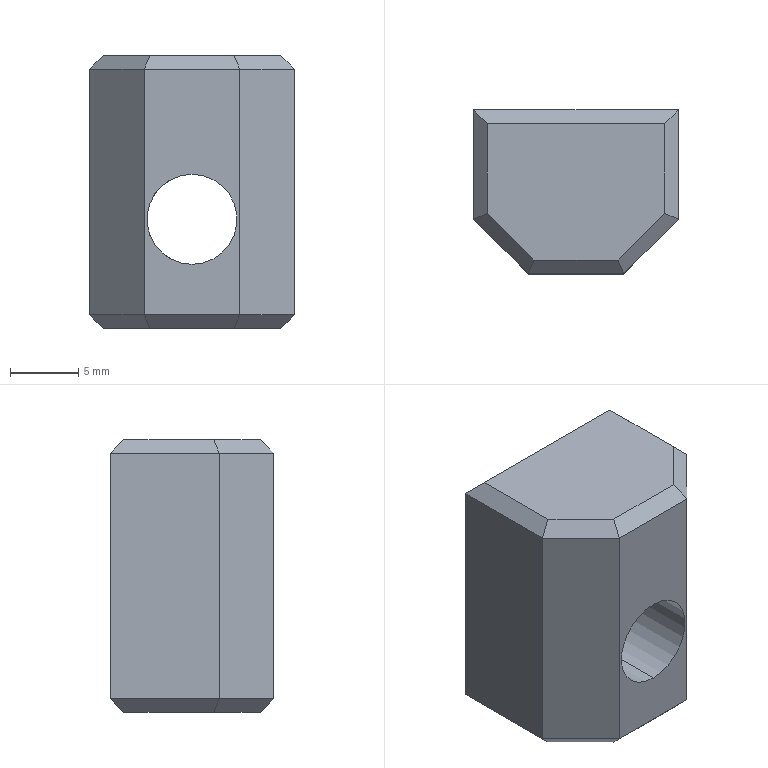Part | Creo | 1 solid | 25 faces | box 15 x 12 x 20 mm | volume 2397 mm3 | plane 21 | cylinder 4 | commonest cylinder face diameters 6.6 x2 11 x2
STEP:
#1=CARTESIAN_POINT('',(0.,0.,0.));
#2=DIRECTION('',(0.,0.,1.));
#3=DIRECTION('',(1.,0.,0.));
#4=AXIS2_PLACEMENT_3D('',#1,#2,#3);
#5=CARTESIAN_POINT('',(-37.05,242.414,-34.767));
#6=VERTEX_POINT('',#5);
#7=CARTESIAN_POINT('',(-40.464,239.,-34.767));
#8=VERTEX_POINT('',#7);
#9=CARTESIAN_POINT('',(-37.05,242.414,-34.767));
#10=DIRECTION('',(-0.7071,-0.7071,0.));
#11=VECTOR('',#10,4.828);
#12=LINE('',#9,#11);
#13=EDGE_CURVE('',#6,#8,#12,.T.);
#14=ORIENTED_EDGE('',*,*,#13,.F.);
#15=CARTESIAN_POINT('',(-37.05,249.,-34.767));
#16=VERTEX_POINT('',#15);
#17=CARTESIAN_POINT('',(-37.05,242.414,-34.767));
#18=DIRECTION('',(0.,1.,0.));
#19=VECTOR('',#18,6.586);
#20=LINE('',#17,#19);
#21=EDGE_CURVE('',#6,#16,#20,.T.);
#22=ORIENTED_EDGE('',*,*,#21,.T.);
#23=CARTESIAN_POINT('',(-50.05,249.,-34.767));
#24=VERTEX_POINT('',#23);
#25=CARTESIAN_POINT('',(-37.05,249.,-34.767));
#26=DIRECTION('',(-1.,0.,0.));
#27=VECTOR('',#26,13.);
#28=LINE('',#25,#27);
#29=EDGE_CURVE('',#16,#24,#28,.T.);
#30=ORIENTED_EDGE('',*,*,#29,.T.);
#31=CARTESIAN_POINT('',(-50.05,242.414,-34.767));
#32=VERTEX_POINT('',#31);
#33=CARTESIAN_POINT('',(-50.05,249.,-34.767));
#34=DIRECTION('',(0.,-1.,0.));
#35=VECTOR('',#34,6.586);
#36=LINE('',#33,#35);
#37=EDGE_CURVE('',#24,#32,#36,.T.);
#38=ORIENTED_EDGE('',*,*,#37,.T.);
#39=CARTESIAN_POINT('',(-46.636,239.,-34.767));
#40=VERTEX_POINT('',#39);
#41=CARTESIAN_POINT('',(-46.636,239.,-34.767));
#42=DIRECTION('',(-0.7071,0.7071,0.));
#43=VECTOR('',#42,4.828);
#44=LINE('',#41,#43);
#45=EDGE_CURVE('',#40,#32,#44,.T.);
#46=ORIENTED_EDGE('',*,*,#45,.F.);
#47=CARTESIAN_POINT('',(-46.636,239.,-34.767));
#48=DIRECTION('',(1.,0.,0.));
#49=VECTOR('',#48,6.172);
#50=LINE('',#47,#49);
#51=EDGE_CURVE('',#40,#8,#50,.T.);
#52=ORIENTED_EDGE('',*,*,#51,.T.);
#53=EDGE_LOOP('',(#14,#22,#30,#38,#46,#52));
#54=FACE_OUTER_BOUND('',#53,.F.);
#55=CARTESIAN_POINT('',(-36.05,250.,-34.767));
#56=DIRECTION('',(0.,0.,-1.));
#57=DIRECTION('',(0.,1.,0.));
#58=AXIS2_PLACEMENT_3D('',#55,#56,#57);
#59=PLANE('',#58);
#60=ADVANCED_FACE('',(#54),#59,.T.);
#61=CARTESIAN_POINT('',(-40.05,238.,-33.767));
#62=VERTEX_POINT('',#61);
#63=CARTESIAN_POINT('',(-40.464,239.,-34.767));
#64=DIRECTION('',(0.2811,-0.6786,0.6786));
#65=VECTOR('',#64,1.474);
#66=LINE('',#63,#65);
#67=EDGE_CURVE('',#8,#62,#66,.T.);
#68=ORIENTED_EDGE('',*,*,#67,.T.);
#69=CARTESIAN_POINT('',(-36.05,242.,-33.767));
#70=VERTEX_POINT('',#69);
#71=CARTESIAN_POINT('',(-36.05,242.,-33.767));
#72=DIRECTION('',(-0.7071,-0.7071,0.));
#73=VECTOR('',#72,5.657);
#74=LINE('',#71,#73);
#75=EDGE_CURVE('',#70,#62,#74,.T.);
#76=ORIENTED_EDGE('',*,*,#75,.F.);
#77=CARTESIAN_POINT('',(-36.05,242.,-33.767));
#78=DIRECTION('',(-0.6786,0.2811,-0.6786));
#79=VECTOR('',#78,1.474);
#80=LINE('',#77,#79);
#81=EDGE_CURVE('',#70,#6,#80,.T.);
#82=ORIENTED_EDGE('',*,*,#81,.T.);
#83=ORIENTED_EDGE('',*,*,#13,.T.);
#84=EDGE_LOOP('',(#68,#76,#82,#83));
#85=FACE_OUTER_BOUND('',#84,.F.);
#86=CARTESIAN_POINT('',(-40.05,238.,-33.767));
#87=DIRECTION('',(0.5,-0.5,-0.7071));
#88=DIRECTION('',(-0.7071,-0.7071,0.));
#89=AXIS2_PLACEMENT_3D('',#86,#87,#88);
#90=PLANE('',#89);
#91=ADVANCED_FACE('',(#85),#90,.T.);
#92=CARTESIAN_POINT('',(-47.05,238.,-33.767));
#93=VERTEX_POINT('',#92);
#94=CARTESIAN_POINT('',(-46.636,239.,-34.767));
#95=DIRECTION('',(-0.2811,-0.6786,0.6786));
#96=VECTOR('',#95,1.474);
#97=LINE('',#94,#96);
#98=EDGE_CURVE('',#40,#93,#97,.T.);
#99=ORIENTED_EDGE('',*,*,#98,.T.);
#100=CARTESIAN_POINT('',(-40.05,238.,-33.767));
#101=DIRECTION('',(-1.,0.,0.));
#102=VECTOR('',#101,7.);
#103=LINE('',#100,#102);
#104=EDGE_CURVE('',#62,#93,#103,.T.);
#105=ORIENTED_EDGE('',*,*,#104,.F.);
#106=ORIENTED_EDGE('',*,*,#67,.F.);
#107=ORIENTED_EDGE('',*,*,#51,.F.);
#108=EDGE_LOOP('',(#99,#105,#106,#107));
#109=FACE_OUTER_BOUND('',#108,.F.);
#110=CARTESIAN_POINT('',(-36.05,239.,-34.767));
#111=DIRECTION('',(0.,0.7071,0.7071));
#112=DIRECTION('',(-1.,0.,0.));
#113=AXIS2_PLACEMENT_3D('',#110,#111,#112);
#114=PLANE('',#113);
#115=ADVANCED_FACE('',(#109),#114,.F.);
#116=CARTESIAN_POINT('',(-51.05,242.,-33.767));
#117=VERTEX_POINT('',#116);
#118=CARTESIAN_POINT('',(-50.05,242.414,-34.767));
#119=DIRECTION('',(-0.6786,-0.2811,0.6786));
#120=VECTOR('',#119,1.474);
#121=LINE('',#118,#120);
#122=EDGE_CURVE('',#32,#117,#121,.T.);
#123=ORIENTED_EDGE('',*,*,#122,.T.);
#124=CARTESIAN_POINT('',(-47.05,238.,-33.767));
#125=DIRECTION('',(-0.7071,0.7071,0.));
#126=VECTOR('',#125,5.657);
#127=LINE('',#124,#126);
#128=EDGE_CURVE('',#93,#117,#127,.T.);
#129=ORIENTED_EDGE('',*,*,#128,.F.);
#130=ORIENTED_EDGE('',*,*,#98,.F.);
#131=ORIENTED_EDGE('',*,*,#45,.T.);
#132=EDGE_LOOP('',(#123,#129,#130,#131));
#133=FACE_OUTER_BOUND('',#132,.F.);
#134=CARTESIAN_POINT('',(-47.05,238.,-33.767));
#135=DIRECTION('',(-0.5,-0.5,-0.7071));
#136=DIRECTION('',(-0.7071,0.7071,0.));
#137=AXIS2_PLACEMENT_3D('',#134,#135,#136);
#138=PLANE('',#137);
#139=ADVANCED_FACE('',(#133),#138,.T.);
#140=CARTESIAN_POINT('',(-51.05,250.,-33.767));
#141=VERTEX_POINT('',#140);
#142=CARTESIAN_POINT('',(-51.05,250.,-33.767));
#143=DIRECTION('',(0.5774,-0.5774,-0.5774));
#144=VECTOR('',#143,1.732);
#145=LINE('',#142,#144);
#146=EDGE_CURVE('',#141,#24,#145,.T.);
#147=ORIENTED_EDGE('',*,*,#146,.F.);
#148=CARTESIAN_POINT('',(-51.05,242.,-33.767));
#149=DIRECTION('',(0.,1.,0.));
#150=VECTOR('',#149,8.);
#151=LINE('',#148,#150);
#152=EDGE_CURVE('',#117,#141,#151,.T.);
#153=ORIENTED_EDGE('',*,*,#152,.F.);
#154=ORIENTED_EDGE('',*,*,#122,.F.);
#155=ORIENTED_EDGE('',*,*,#37,.F.);
#156=EDGE_LOOP('',(#147,#153,#154,#155));
#157=FACE_OUTER_BOUND('',#156,.F.);
#158=CARTESIAN_POINT('',(-51.05,250.,-33.767));
#159=DIRECTION('',(0.7071,0.,0.7071));
#160=DIRECTION('',(0.,-1.,0.));
#161=AXIS2_PLACEMENT_3D('',#158,#159,#160);
#162=PLANE('',#161);
#163=ADVANCED_FACE('',(#157),#162,.F.);
#164=ORIENTED_EDGE('',*,*,#146,.T.);
#165=ORIENTED_EDGE('',*,*,#29,.F.);
#166=CARTESIAN_POINT('',(-36.05,250.,-33.767));
#167=VERTEX_POINT('',#166);
#168=CARTESIAN_POINT('',(-36.05,250.,-33.767));
#169=DIRECTION('',(-0.5774,-0.5774,-0.5774));
#170=VECTOR('',#169,1.732);
#171=LINE('',#168,#170);
#172=EDGE_CURVE('',#167,#16,#171,.T.);
#173=ORIENTED_EDGE('',*,*,#172,.F.);
#174=CARTESIAN_POINT('',(-51.05,250.,-33.767));
#175=DIRECTION('',(1.,0.,0.));
#176=VECTOR('',#175,15.);
#177=LINE('',#174,#176);
#178=EDGE_CURVE('',#141,#167,#177,.T.);
#179=ORIENTED_EDGE('',*,*,#178,.F.);
#180=EDGE_LOOP('',(#164,#165,#173,#179));
#181=FACE_OUTER_BOUND('',#180,.F.);
#182=CARTESIAN_POINT('',(50.05,250.,-33.767));
#183=DIRECTION('',(0.,0.7071,-0.7071));
#184=DIRECTION('',(1.,0.,0.));
#185=AXIS2_PLACEMENT_3D('',#182,#183,#184);
#186=PLANE('',#185);
#187=ADVANCED_FACE('',(#181),#186,.T.);
#188=ORIENTED_EDGE('',*,*,#172,.T.);
#189=ORIENTED_EDGE('',*,*,#21,.F.);
#190=ORIENTED_EDGE('',*,*,#81,.F.);
#191=CARTESIAN_POINT('',(-36.05,250.,-33.767));
#192=DIRECTION('',(0.,-1.,0.));
#193=VECTOR('',#192,8.);
#194=LINE('',#191,#193);
#195=EDGE_CURVE('',#167,#70,#194,.T.);
#196=ORIENTED_EDGE('',*,*,#195,.F.);
#197=EDGE_LOOP('',(#188,#189,#190,#196));
#198=FACE_OUTER_BOUND('',#197,.F.);
#199=CARTESIAN_POINT('',(-37.05,250.,-34.767));
#200=DIRECTION('',(-0.7071,0.,0.7071));
#201=DIRECTION('',(0.,-1.,0.));
#202=AXIS2_PLACEMENT_3D('',#199,#200,#201);
#203=PLANE('',#202);
#204=ADVANCED_FACE('',(#198),#203,.F.);
#205=CARTESIAN_POINT('',(-36.05,242.,-15.767));
#206=VERTEX_POINT('',#205);
#207=CARTESIAN_POINT('',(-36.05,242.,-15.767));
#208=DIRECTION('',(0.,0.,-1.));
#209=VECTOR('',#208,18.);
#210=LINE('',#207,#209);
#211=EDGE_CURVE('',#206,#70,#210,.T.);
#212=ORIENTED_EDGE('',*,*,#211,.F.);
#213=CARTESIAN_POINT('',(-36.05,250.,-15.767));
#214=VERTEX_POINT('',#213);
#215=CARTESIAN_POINT('',(-36.05,242.,-15.767));
#216=DIRECTION('',(0.,1.,0.));
#217=VECTOR('',#216,8.);
#218=LINE('',#215,#217);
#219=EDGE_CURVE('',#206,#214,#218,.T.);
#220=ORIENTED_EDGE('',*,*,#219,.T.);
#221=CARTESIAN_POINT('',(-36.05,250.,-33.767));
#222=DIRECTION('',(0.,0.,1.));
#223=VECTOR('',#222,18.);
#224=LINE('',#221,#223);
#225=EDGE_CURVE('',#167,#214,#224,.T.);
#226=ORIENTED_EDGE('',*,*,#225,.F.);
#227=ORIENTED_EDGE('',*,*,#195,.T.);
#228=EDGE_LOOP('',(#212,#220,#226,#227));
#229=FACE_OUTER_BOUND('',#228,.F.);
#230=CARTESIAN_POINT('',(-36.05,250.,-14.767));
#231=DIRECTION('',(1.,0.,0.));
#232=DIRECTION('',(0.,0.,-1.));
#233=AXIS2_PLACEMENT_3D('',#230,#231,#232);
#234=PLANE('',#233);
#235=ADVANCED_FACE('',(#229),#234,.T.);
#236=ORIENTED_EDGE('',*,*,#211,.T.);
#237=ORIENTED_EDGE('',*,*,#75,.T.);
#238=CARTESIAN_POINT('',(-40.05,238.,-15.767));
#239=VERTEX_POINT('',#238);
#240=CARTESIAN_POINT('',(-40.05,238.,-33.767));
#241=DIRECTION('',(0.,0.,1.));
#242=VECTOR('',#241,18.);
#243=LINE('',#240,#242);
#244=EDGE_CURVE('',#62,#239,#243,.T.);
#245=ORIENTED_EDGE('',*,*,#244,.T.);
#246=CARTESIAN_POINT('',(-40.05,238.,-15.767));
#247=DIRECTION('',(0.7071,0.7071,0.));
#248=VECTOR('',#247,5.657);
#249=LINE('',#246,#248);
#250=EDGE_CURVE('',#239,#206,#249,.T.);
#251=ORIENTED_EDGE('',*,*,#250,.T.);
#252=EDGE_LOOP('',(#236,#237,#245,#251));
#253=FACE_OUTER_BOUND('',#252,.F.);
#254=CARTESIAN_POINT('',(-40.05,238.,8.06));
#255=DIRECTION('',(-0.7071,0.7071,0.));
#256=DIRECTION('',(0.,0.,-1.));
#257=AXIS2_PLACEMENT_3D('',#254,#255,#256);
#258=PLANE('',#257);
#259=ADVANCED_FACE('',(#253),#258,.F.);
#260=ORIENTED_EDGE('',*,*,#244,.F.);
#261=ORIENTED_EDGE('',*,*,#104,.T.);
#262=CARTESIAN_POINT('',(-47.05,238.,-15.767));
#263=VERTEX_POINT('',#262);
#264=CARTESIAN_POINT('',(-47.05,238.,-15.767));
#265=DIRECTION('',(0.,0.,-1.));
#266=VECTOR('',#265,18.);
#267=LINE('',#264,#266);
#268=EDGE_CURVE('',#263,#93,#267,.T.);
#269=ORIENTED_EDGE('',*,*,#268,.F.);
#270=CARTESIAN_POINT('',(-47.05,238.,-15.767));
#271=DIRECTION('',(1.,0.,0.));
#272=VECTOR('',#271,7.);
#273=LINE('',#270,#272);
#274=EDGE_CURVE('',#263,#239,#273,.T.);
#275=ORIENTED_EDGE('',*,*,#274,.T.);
#276=EDGE_LOOP('',(#260,#261,#269,#275));
#277=FACE_OUTER_BOUND('',#276,.F.);
#278=CARTESIAN_POINT('',(-43.55,238.,-30.067));
#279=VERTEX_POINT('',#278);
#280=CARTESIAN_POINT('',(-43.55,238.,-23.467));
#281=VERTEX_POINT('',#280);
#282=CARTESIAN_POINT('',(-43.55,238.,-26.767));
#283=DIRECTION('',(0.,1.,0.));
#284=DIRECTION('',(0.,0.,-1.));
#285=AXIS2_PLACEMENT_3D('',#282,#283,#284);
#286=CIRCLE('',#285,3.3);
#287=EDGE_CURVE('',#279,#281,#286,.T.);
#288=ORIENTED_EDGE('',*,*,#287,.F.);
#289=CARTESIAN_POINT('',(-43.55,238.,-26.767));
#290=DIRECTION('',(0.,1.,0.));
#291=DIRECTION('',(0.,0.,1.));
#292=AXIS2_PLACEMENT_3D('',#289,#290,#291);
#293=CIRCLE('',#292,3.3);
#294=EDGE_CURVE('',#281,#279,#293,.T.);
#295=ORIENTED_EDGE('',*,*,#294,.F.);
#296=EDGE_LOOP('',(#288,#295));
#297=FACE_BOUND('',#296,.F.);
#298=CARTESIAN_POINT('',(50.05,238.,8.06));
#299=DIRECTION('',(0.,-1.,0.));
#300=DIRECTION('',(0.,0.,-1.));
#301=AXIS2_PLACEMENT_3D('',#298,#299,#300);
#302=PLANE('',#301);
#303=ADVANCED_FACE('',(#277,#297),#302,.T.);
#304=CARTESIAN_POINT('',(-43.55,243.,-23.467));
#305=VERTEX_POINT('',#304);
#306=CARTESIAN_POINT('',(-46.85,243.,-26.767));
#307=VERTEX_POINT('',#306);
#308=CARTESIAN_POINT('',(-43.55,243.,-26.767));
#309=DIRECTION('',(0.,-1.,0.));
#310=DIRECTION('',(0.,0.,1.));
#311=AXIS2_PLACEMENT_3D('',#308,#309,#310);
#312=CIRCLE('',#311,3.3);
#313=EDGE_CURVE('',#305,#307,#312,.T.);
#314=ORIENTED_EDGE('',*,*,#313,.T.);
#315=CARTESIAN_POINT('',(-43.55,243.,-30.067));
#316=VERTEX_POINT('',#315);
#317=CARTESIAN_POINT('',(-43.55,243.,-26.767));
#318=DIRECTION('',(0.,-1.,0.));
#319=DIRECTION('',(-1.,0.,0.));
#320=AXIS2_PLACEMENT_3D('',#317,#318,#319);
#321=CIRCLE('',#320,3.3);
#322=EDGE_CURVE('',#307,#316,#321,.T.);
#323=ORIENTED_EDGE('',*,*,#322,.T.);
#324=CARTESIAN_POINT('',(-43.55,243.,-30.067));
#325=DIRECTION('',(0.,-1.,0.));
#326=VECTOR('',#325,5.);
#327=LINE('',#324,#326);
#328=EDGE_CURVE('',#316,#279,#327,.T.);
#329=ORIENTED_EDGE('',*,*,#328,.T.);
#330=ORIENTED_EDGE('',*,*,#287,.T.);
#331=CARTESIAN_POINT('',(-43.55,243.,-23.467));
#332=DIRECTION('',(0.,-1.,0.));
#333=VECTOR('',#332,5.);
#334=LINE('',#331,#333);
#335=EDGE_CURVE('',#305,#281,#334,.T.);
#336=ORIENTED_EDGE('',*,*,#335,.F.);
#337=EDGE_LOOP('',(#314,#323,#329,#330,#336));
#338=FACE_OUTER_BOUND('',#337,.F.);
#339=CARTESIAN_POINT('',(-43.55,50.,-26.767));
#340=DIRECTION('',(0.,-1.,0.));
#341=DIRECTION('',(0.,0.,-1.));
#342=AXIS2_PLACEMENT_3D('',#339,#340,#341);
#343=CYLINDRICAL_SURFACE('',#342,3.3);
#344=ADVANCED_FACE('',(#338),#343,.F.);
#345=CARTESIAN_POINT('',(-49.05,243.,-26.767));
#346=VERTEX_POINT('',#345);
#347=CARTESIAN_POINT('',(-43.55,243.,-21.267));
#348=VERTEX_POINT('',#347);
#349=CARTESIAN_POINT('',(-43.55,243.,-26.767));
#350=DIRECTION('',(0.,1.,0.));
#351=DIRECTION('',(-1.,0.,0.));
#352=AXIS2_PLACEMENT_3D('',#349,#350,#351);
#353=CIRCLE('',#352,5.5);
#354=EDGE_CURVE('',#346,#348,#353,.T.);
#355=ORIENTED_EDGE('',*,*,#354,.F.);
#356=CARTESIAN_POINT('',(-43.55,243.,-32.267));
#357=VERTEX_POINT('',#356);
#358=CARTESIAN_POINT('',(-43.55,243.,-26.767));
#359=DIRECTION('',(0.,1.,0.));
#360=DIRECTION('',(0.,0.,-1.));
#361=AXIS2_PLACEMENT_3D('',#358,#359,#360);
#362=CIRCLE('',#361,5.5);
#363=EDGE_CURVE('',#357,#346,#362,.T.);
#364=ORIENTED_EDGE('',*,*,#363,.F.);
#365=CARTESIAN_POINT('',(-38.05,243.,-26.767));
#366=VERTEX_POINT('',#365);
#367=CARTESIAN_POINT('',(-43.55,243.,-26.767));
#368=DIRECTION('',(0.,1.,0.));
#369=DIRECTION('',(1.,0.,0.));
#370=AXIS2_PLACEMENT_3D('',#367,#368,#369);
#371=CIRCLE('',#370,5.5);
#372=EDGE_CURVE('',#366,#357,#371,.T.);
#373=ORIENTED_EDGE('',*,*,#372,.F.);
#374=CARTESIAN_POINT('',(-43.55,243.,-26.767));
#375=DIRECTION('',(0.,1.,0.));
#376=DIRECTION('',(0.,0.,1.));
#377=AXIS2_PLACEMENT_3D('',#374,#375,#376);
#378=CIRCLE('',#377,5.5);
#379=EDGE_CURVE('',#348,#366,#378,.T.);
#380=ORIENTED_EDGE('',*,*,#379,.F.);
#381=EDGE_LOOP('',(#355,#364,#373,#380));
#382=FACE_OUTER_BOUND('',#381,.F.);
#383=ORIENTED_EDGE('',*,*,#322,.F.);
#384=ORIENTED_EDGE('',*,*,#313,.F.);
#385=CARTESIAN_POINT('',(-43.55,243.,-26.767));
#386=DIRECTION('',(0.,-1.,0.));
#387=DIRECTION('',(0.,0.,-1.));
#388=AXIS2_PLACEMENT_3D('',#385,#386,#387);
#389=CIRCLE('',#388,3.3);
#390=EDGE_CURVE('',#316,#305,#389,.T.);
#391=ORIENTED_EDGE('',*,*,#390,.F.);
#392=EDGE_LOOP('',(#383,#384,#391));
#393=FACE_BOUND('',#392,.F.);
#394=CARTESIAN_POINT('',(-43.55,243.,-21.267));
#395=DIRECTION('',(0.,-1.,0.));
#396=DIRECTION('',(1.,0.,0.));
#397=AXIS2_PLACEMENT_3D('',#394,#395,#396);
#398=PLANE('',#397);
#399=ADVANCED_FACE('',(#382,#393),#398,.F.);
#400=ORIENTED_EDGE('',*,*,#390,.T.);
#401=ORIENTED_EDGE('',*,*,#335,.T.);
#402=ORIENTED_EDGE('',*,*,#294,.T.);
#403=ORIENTED_EDGE('',*,*,#328,.F.);
#404=EDGE_LOOP('',(#400,#401,#402,#403));
#405=FACE_OUTER_BOUND('',#404,.F.);
#406=CARTESIAN_POINT('',(-43.55,50.,-26.767));
#407=DIRECTION('',(0.,-1.,0.));
#408=DIRECTION('',(0.,0.,-1.));
#409=AXIS2_PLACEMENT_3D('',#406,#407,#408);
#410=CYLINDRICAL_SURFACE('',#409,3.3);
#411=ADVANCED_FACE('',(#405),#410,.F.);
#412=CARTESIAN_POINT('',(-43.55,250.,-21.267));
#413=VERTEX_POINT('',#412);
#414=CARTESIAN_POINT('',(-43.55,250.,-32.267));
#415=VERTEX_POINT('',#414);
#416=CARTESIAN_POINT('',(-43.55,250.,-26.767));
#417=DIRECTION('',(0.,-1.,0.));
#418=DIRECTION('',(0.,0.,1.));
#419=AXIS2_PLACEMENT_3D('',#416,#417,#418);
#420=CIRCLE('',#419,5.5);
#421=EDGE_CURVE('',#413,#415,#420,.T.);
#422=ORIENTED_EDGE('',*,*,#421,.T.);
#423=CARTESIAN_POINT('',(-43.55,250.,-32.267));
#424=DIRECTION('',(0.,-1.,0.));
#425=VECTOR('',#424,7.);
#426=LINE('',#423,#425);
#427=EDGE_CURVE('',#415,#357,#426,.T.);
#428=ORIENTED_EDGE('',*,*,#427,.T.);
#429=ORIENTED_EDGE('',*,*,#363,.T.);
#430=ORIENTED_EDGE('',*,*,#354,.T.);
#431=CARTESIAN_POINT('',(-43.55,250.,-21.267));
#432=DIRECTION('',(0.,-1.,0.));
#433=VECTOR('',#432,7.);
#434=LINE('',#431,#433);
#435=EDGE_CURVE('',#413,#348,#434,.T.);
#436=ORIENTED_EDGE('',*,*,#435,.F.);
#437=EDGE_LOOP('',(#422,#428,#429,#430,#436));
#438=FACE_OUTER_BOUND('',#437,.F.);
#439=CARTESIAN_POINT('',(-43.55,250.,-26.767));
#440=DIRECTION('',(0.,-1.,0.));
#441=DIRECTION('',(0.,0.,-1.));
#442=AXIS2_PLACEMENT_3D('',#439,#440,#441);
#443=CYLINDRICAL_SURFACE('',#442,5.5);
#444=ADVANCED_FACE('',(#438),#443,.F.);
#445=CARTESIAN_POINT('',(-51.05,250.,-15.767));
#446=VERTEX_POINT('',#445);
#447=CARTESIAN_POINT('',(-51.05,250.,-15.767));
#448=DIRECTION('',(0.,0.,-1.));
#449=VECTOR('',#448,18.);
#450=LINE('',#447,#449);
#451=EDGE_CURVE('',#446,#141,#450,.T.);
#452=ORIENTED_EDGE('',*,*,#451,.T.);
#453=ORIENTED_EDGE('',*,*,#178,.T.);
#454=ORIENTED_EDGE('',*,*,#225,.T.);
#455=CARTESIAN_POINT('',(-36.05,250.,-15.767));
#456=DIRECTION('',(-1.,0.,0.));
#457=VECTOR('',#456,15.);
#458=LINE('',#455,#457);
#459=EDGE_CURVE('',#214,#446,#458,.T.);
#460=ORIENTED_EDGE('',*,*,#459,.T.);
#461=EDGE_LOOP('',(#452,#453,#454,#460));
#462=FACE_OUTER_BOUND('',#461,.F.);
#463=CARTESIAN_POINT('',(-43.55,250.,-26.767));
#464=DIRECTION('',(0.,-1.,0.));
#465=DIRECTION('',(0.,0.,-1.));
#466=AXIS2_PLACEMENT_3D('',#463,#464,#465);
#467=CIRCLE('',#466,5.5);
#468=EDGE_CURVE('',#415,#413,#467,.T.);
#469=ORIENTED_EDGE('',*,*,#468,.F.);
#470=ORIENTED_EDGE('',*,*,#421,.F.);
#471=EDGE_LOOP('',(#469,#470));
#472=FACE_BOUND('',#471,.F.);
#473=CARTESIAN_POINT('',(50.05,250.,8.06));
#474=DIRECTION('',(0.,-1.,0.));
#475=DIRECTION('',(0.,0.,-1.));
#476=AXIS2_PLACEMENT_3D('',#473,#474,#475);
#477=PLANE('',#476);
#478=ADVANCED_FACE('',(#462,#472),#477,.F.);
#479=ORIENTED_EDGE('',*,*,#468,.T.);
#480=ORIENTED_EDGE('',*,*,#435,.T.);
#481=ORIENTED_EDGE('',*,*,#379,.T.);
#482=ORIENTED_EDGE('',*,*,#372,.T.);
#483=ORIENTED_EDGE('',*,*,#427,.F.);
#484=EDGE_LOOP('',(#479,#480,#481,#482,#483));
#485=FACE_OUTER_BOUND('',#484,.F.);
#486=CARTESIAN_POINT('',(-43.55,250.,-26.767));
#487=DIRECTION('',(0.,-1.,0.));
#488=DIRECTION('',(0.,0.,-1.));
#489=AXIS2_PLACEMENT_3D('',#486,#487,#488);
#490=CYLINDRICAL_SURFACE('',#489,5.5);
#491=ADVANCED_FACE('',(#485),#490,.F.);
#492=ORIENTED_EDGE('',*,*,#451,.F.);
#493=CARTESIAN_POINT('',(-51.05,242.,-15.767));
#494=VERTEX_POINT('',#493);
#495=CARTESIAN_POINT('',(-51.05,250.,-15.767));
#496=DIRECTION('',(0.,-1.,0.));
#497=VECTOR('',#496,8.);
#498=LINE('',#495,#497);
#499=EDGE_CURVE('',#446,#494,#498,.T.);
#500=ORIENTED_EDGE('',*,*,#499,.T.);
#501=CARTESIAN_POINT('',(-51.05,242.,-33.767));
#502=DIRECTION('',(0.,0.,1.));
#503=VECTOR('',#502,18.);
#504=LINE('',#501,#503);
#505=EDGE_CURVE('',#117,#494,#504,.T.);
#506=ORIENTED_EDGE('',*,*,#505,.F.);
#507=ORIENTED_EDGE('',*,*,#152,.T.);
#508=EDGE_LOOP('',(#492,#500,#506,#507));
#509=FACE_OUTER_BOUND('',#508,.F.);
#510=CARTESIAN_POINT('',(-51.05,250.,-34.767));
#511=DIRECTION('',(-1.,0.,0.));
#512=DIRECTION('',(0.,0.,1.));
#513=AXIS2_PLACEMENT_3D('',#510,#511,#512);
#514=PLANE('',#513);
#515=ADVANCED_FACE('',(#509),#514,.T.);
#516=CARTESIAN_POINT('',(-50.05,242.414,-14.767));
#517=VERTEX_POINT('',#516);
#518=CARTESIAN_POINT('',(-51.05,242.,-15.767));
#519=DIRECTION('',(0.6786,0.2811,0.6786));
#520=VECTOR('',#519,1.474);
#521=LINE('',#518,#520);
#522=EDGE_CURVE('',#494,#517,#521,.T.);
#523=ORIENTED_EDGE('',*,*,#522,.F.);
#524=ORIENTED_EDGE('',*,*,#499,.F.);
#525=CARTESIAN_POINT('',(-50.05,249.,-14.767));
#526=VERTEX_POINT('',#525);
#527=CARTESIAN_POINT('',(-50.05,249.,-14.767));
#528=DIRECTION('',(-0.5774,0.5774,-0.5774));
#529=VECTOR('',#528,1.732);
#530=LINE('',#527,#529);
#531=EDGE_CURVE('',#526,#446,#530,.T.);
#532=ORIENTED_EDGE('',*,*,#531,.F.);
#533=CARTESIAN_POINT('',(-50.05,242.414,-14.767));
#534=DIRECTION('',(0.,1.,0.));
#535=VECTOR('',#534,6.586);
#536=LINE('',#533,#535);
#537=EDGE_CURVE('',#517,#526,#536,.T.);
#538=ORIENTED_EDGE('',*,*,#537,.F.);
#539=EDGE_LOOP('',(#523,#524,#532,#538));
#540=FACE_OUTER_BOUND('',#539,.F.);
#541=CARTESIAN_POINT('',(-50.05,250.,-14.767));
#542=DIRECTION('',(0.7071,0.,-0.7071));
#543=DIRECTION('',(0.,-1.,0.));
#544=AXIS2_PLACEMENT_3D('',#541,#542,#543);
#545=PLANE('',#544);
#546=ADVANCED_FACE('',(#540),#545,.F.);
#547=ORIENTED_EDGE('',*,*,#522,.T.);
#548=CARTESIAN_POINT('',(-46.636,239.,-14.767));
#549=VERTEX_POINT('',#548);
#550=CARTESIAN_POINT('',(-50.05,242.414,-14.767));
#551=DIRECTION('',(0.7071,-0.7071,0.));
#552=VECTOR('',#551,4.828);
#553=LINE('',#550,#552);
#554=EDGE_CURVE('',#517,#549,#553,.T.);
#555=ORIENTED_EDGE('',*,*,#554,.T.);
#556=CARTESIAN_POINT('',(-47.05,238.,-15.767));
#557=DIRECTION('',(0.2811,0.6786,0.6786));
#558=VECTOR('',#557,1.474);
#559=LINE('',#556,#558);
#560=EDGE_CURVE('',#263,#549,#559,.T.);
#561=ORIENTED_EDGE('',*,*,#560,.F.);
#562=CARTESIAN_POINT('',(-51.05,242.,-15.767));
#563=DIRECTION('',(0.7071,-0.7071,0.));
#564=VECTOR('',#563,5.657);
#565=LINE('',#562,#564);
#566=EDGE_CURVE('',#494,#263,#565,.T.);
#567=ORIENTED_EDGE('',*,*,#566,.F.);
#568=EDGE_LOOP('',(#547,#555,#561,#567));
#569=FACE_OUTER_BOUND('',#568,.F.);
#570=CARTESIAN_POINT('',(-47.05,238.,-15.767));
#571=DIRECTION('',(-0.5,-0.5,0.7071));
#572=DIRECTION('',(0.7071,-0.7071,0.));
#573=AXIS2_PLACEMENT_3D('',#570,#571,#572);
#574=PLANE('',#573);
#575=ADVANCED_FACE('',(#569),#574,.T.);
#576=CARTESIAN_POINT('',(-40.464,239.,-14.767));
#577=VERTEX_POINT('',#576);
#578=CARTESIAN_POINT('',(-37.05,242.414,-14.767));
#579=VERTEX_POINT('',#578);
#580=CARTESIAN_POINT('',(-40.464,239.,-14.767));
#581=DIRECTION('',(0.7071,0.7071,0.));
#582=VECTOR('',#581,4.828);
#583=LINE('',#580,#582);
#584=EDGE_CURVE('',#577,#579,#583,.T.);
#585=ORIENTED_EDGE('',*,*,#584,.F.);
#586=CARTESIAN_POINT('',(-40.464,239.,-14.767));
#587=DIRECTION('',(-1.,0.,0.));
#588=VECTOR('',#587,6.172);
#589=LINE('',#586,#588);
#590=EDGE_CURVE('',#577,#549,#589,.T.);
#591=ORIENTED_EDGE('',*,*,#590,.T.);
#592=ORIENTED_EDGE('',*,*,#554,.F.);
#593=ORIENTED_EDGE('',*,*,#537,.T.);
#594=CARTESIAN_POINT('',(-37.05,249.,-14.767));
#595=VERTEX_POINT('',#594);
#596=CARTESIAN_POINT('',(-50.05,249.,-14.767));
#597=DIRECTION('',(1.,0.,0.));
#598=VECTOR('',#597,13.);
#599=LINE('',#596,#598);
#600=EDGE_CURVE('',#526,#595,#599,.T.);
#601=ORIENTED_EDGE('',*,*,#600,.T.);
#602=CARTESIAN_POINT('',(-37.05,249.,-14.767));
#603=DIRECTION('',(0.,-1.,0.));
#604=VECTOR('',#603,6.586);
#605=LINE('',#602,#604);
#606=EDGE_CURVE('',#595,#579,#605,.T.);
#607=ORIENTED_EDGE('',*,*,#606,.T.);
#608=EDGE_LOOP('',(#585,#591,#592,#593,#601,#607));
#609=FACE_OUTER_BOUND('',#608,.F.);
#610=CARTESIAN_POINT('',(-51.05,250.,-14.767));
#611=DIRECTION('',(0.,0.,1.));
#612=DIRECTION('',(1.,0.,0.));
#613=AXIS2_PLACEMENT_3D('',#610,#611,#612);
#614=PLANE('',#613);
#615=ADVANCED_FACE('',(#609),#614,.T.);
#616=CARTESIAN_POINT('',(-37.05,242.414,-14.767));
#617=DIRECTION('',(0.6786,-0.2811,-0.6786));
#618=VECTOR('',#617,1.474);
#619=LINE('',#616,#618);
#620=EDGE_CURVE('',#579,#206,#619,.T.);
#621=ORIENTED_EDGE('',*,*,#620,.T.);
#622=ORIENTED_EDGE('',*,*,#250,.F.);
#623=CARTESIAN_POINT('',(-40.05,238.,-15.767));
#624=DIRECTION('',(-0.2811,0.6786,0.6786));
#625=VECTOR('',#624,1.474);
#626=LINE('',#623,#625);
#627=EDGE_CURVE('',#239,#577,#626,.T.);
#628=ORIENTED_EDGE('',*,*,#627,.T.);
#629=ORIENTED_EDGE('',*,*,#584,.T.);
#630=EDGE_LOOP('',(#621,#622,#628,#629));
#631=FACE_OUTER_BOUND('',#630,.F.);
#632=CARTESIAN_POINT('',(-40.05,238.,-15.767));
#633=DIRECTION('',(0.5,-0.5,0.7071));
#634=DIRECTION('',(0.7071,0.7071,0.));
#635=AXIS2_PLACEMENT_3D('',#632,#633,#634);
#636=PLANE('',#635);
#637=ADVANCED_FACE('',(#631),#636,.T.);
#638=CARTESIAN_POINT('',(-37.05,249.,-14.767));
#639=DIRECTION('',(0.5774,0.5774,-0.5774));
#640=VECTOR('',#639,1.732);
#641=LINE('',#638,#640);
#642=EDGE_CURVE('',#595,#214,#641,.T.);
#643=ORIENTED_EDGE('',*,*,#642,.T.);
#644=ORIENTED_EDGE('',*,*,#219,.F.);
#645=ORIENTED_EDGE('',*,*,#620,.F.);
#646=ORIENTED_EDGE('',*,*,#606,.F.);
#647=EDGE_LOOP('',(#643,#644,#645,#646));
#648=FACE_OUTER_BOUND('',#647,.F.);
#649=CARTESIAN_POINT('',(-36.05,250.,-15.767));
#650=DIRECTION('',(-0.7071,0.,-0.7071));
#651=DIRECTION('',(0.,-1.,0.));
#652=AXIS2_PLACEMENT_3D('',#649,#650,#651);
#653=PLANE('',#652);
#654=ADVANCED_FACE('',(#648),#653,.F.);
#655=ORIENTED_EDGE('',*,*,#531,.T.);
#656=ORIENTED_EDGE('',*,*,#459,.F.);
#657=ORIENTED_EDGE('',*,*,#642,.F.);
#658=ORIENTED_EDGE('',*,*,#600,.F.);
#659=EDGE_LOOP('',(#655,#656,#657,#658));
#660=FACE_OUTER_BOUND('',#659,.F.);
#661=CARTESIAN_POINT('',(50.05,250.,-15.767));
#662=DIRECTION('',(0.,0.7071,0.7071));
#663=DIRECTION('',(-1.,0.,0.));
#664=AXIS2_PLACEMENT_3D('',#661,#662,#663);
#665=PLANE('',#664);
#666=ADVANCED_FACE('',(#660),#665,.T.);
#667=ORIENTED_EDGE('',*,*,#560,.T.);
#668=ORIENTED_EDGE('',*,*,#590,.F.);
#669=ORIENTED_EDGE('',*,*,#627,.F.);
#670=ORIENTED_EDGE('',*,*,#274,.F.);
#671=EDGE_LOOP('',(#667,#668,#669,#670));
#672=FACE_OUTER_BOUND('',#671,.F.);
#673=CARTESIAN_POINT('',(-51.05,239.,-14.767));
#674=DIRECTION('',(0.,0.7071,-0.7071));
#675=DIRECTION('',(1.,0.,0.));
#676=AXIS2_PLACEMENT_3D('',#673,#674,#675);
#677=PLANE('',#676);
#678=ADVANCED_FACE('',(#672),#677,.F.);
#679=ORIENTED_EDGE('',*,*,#505,.T.);
#680=ORIENTED_EDGE('',*,*,#566,.T.);
#681=ORIENTED_EDGE('',*,*,#268,.T.);
#682=ORIENTED_EDGE('',*,*,#128,.T.);
#683=EDGE_LOOP('',(#679,#680,#681,#682));
#684=FACE_OUTER_BOUND('',#683,.F.);
#685=CARTESIAN_POINT('',(-47.05,238.,8.06));
#686=DIRECTION('',(0.7071,0.7071,0.));
#687=DIRECTION('',(0.,0.,1.));
#688=AXIS2_PLACEMENT_3D('',#685,#686,#687);
#689=PLANE('',#688);
#690=ADVANCED_FACE('',(#684),#689,.F.);
#691=CLOSED_SHELL('',(#60,#91,#115,#139,#163,#187,#204,#235,#259,#303,#344,#399,#411,#444,#478,#491,#515,#546,#575,#615,#637,#654,#666,#678,#690));
#692=MANIFOLD_SOLID_BREP('',#691);
#693=(LENGTH_UNIT()NAMED_UNIT(*)SI_UNIT(.MILLI.,.METRE.));
#694=UNCERTAINTY_MEASURE_WITH_UNIT(LENGTH_MEASURE(0.002773),#693,'','');
#695=(NAMED_UNIT(*)PLANE_ANGLE_UNIT()SI_UNIT($,.RADIAN.));
#696=PLANE_ANGLE_MEASURE_WITH_UNIT(PLANE_ANGLE_MEASURE(0.01745),#695);
#697=(CONVERSION_BASED_UNIT('DEGREE',#696)NAMED_UNIT(*)PLANE_ANGLE_UNIT());
#698=(NAMED_UNIT(*)SI_UNIT($,.STERADIAN.)SOLID_ANGLE_UNIT());
#699=(GEOMETRIC_REPRESENTATION_CONTEXT(3)GLOBAL_UNCERTAINTY_ASSIGNED_CONTEXT((#694))GLOBAL_UNIT_ASSIGNED_CONTEXT((#693,#697,#698))REPRESENTATION_CONTEXT('',''));
#700=ADVANCED_BREP_SHAPE_REPRESENTATION('',(#4,#692),#699);